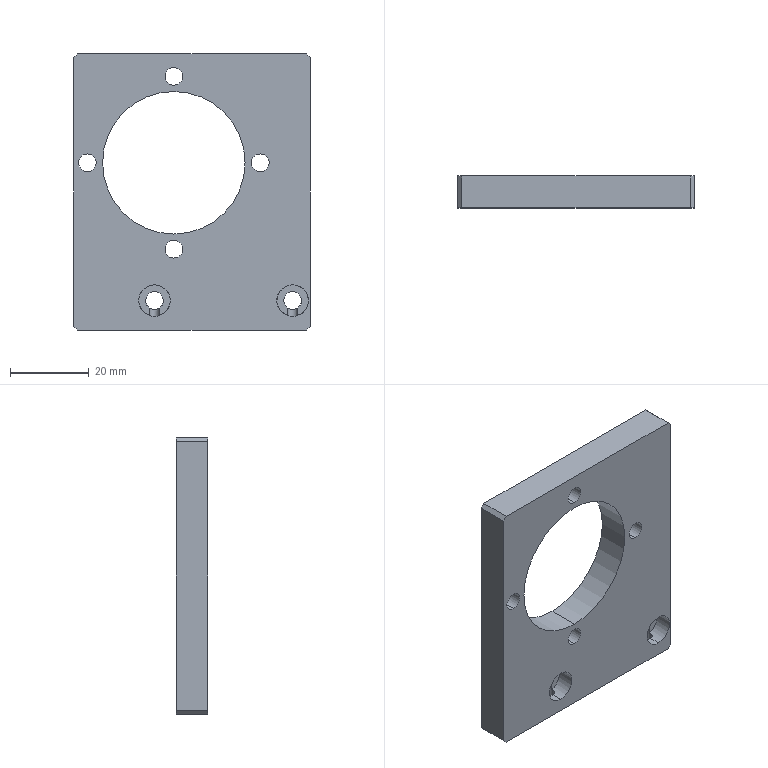Part | STEP file | 08-19 rotary cylinder mounting plate | 1 solid | 34 faces | box 60 x 8 x 70 mm | volume 24290 mm3 | cylinder 22 | plane 12 | commonest cylinder face diameters 4.5 x12 2.5 x4 8 x4 36.1 x2
STEP:
#1=CARTESIAN_POINT('',(26.75,0.,-31.3));
#2=VERTEX_POINT('',#1);
#3=CARTESIAN_POINT('',(25.5,-1.25,-31.5));
#4=VERTEX_POINT('',#3);
#5=CARTESIAN_POINT('',(26.75,0.,-31.3));
#6=CARTESIAN_POINT('',(26.75,-0.1662,-31.3));
#7=CARTESIAN_POINT('',(26.717,-0.3296,-31.311));
#8=CARTESIAN_POINT('',(26.591,-0.6317,-31.349));
#9=CARTESIAN_POINT('',(26.498,-0.7698,-31.375));
#10=CARTESIAN_POINT('',(26.269,-0.9987,-31.427));
#11=CARTESIAN_POINT('',(26.13,-1.092,-31.453));
#12=CARTESIAN_POINT('',(25.83,-1.217,-31.489));
#13=CARTESIAN_POINT('',(25.664,-1.25,-31.5));
#14=CARTESIAN_POINT('',(25.5,-1.25,-31.5));
#15=B_SPLINE_CURVE_WITH_KNOTS('',3,(#5,#6,#7,#8,#9,#10,#11,#12,#13,#14),.UNSPECIFIED.,.F.,.F.,(4,2,2,2,4),(0.0004059,0.0008978,0.00139,0.001882,0.002374),.UNSPECIFIED.);
#16=EDGE_CURVE('',#2,#4,#15,.T.);
#17=ORIENTED_EDGE('',*,*,#16,.F.);
#18=CARTESIAN_POINT('',(26.75,0.,-35.));
#19=VERTEX_POINT('',#18);
#20=CARTESIAN_POINT('',(26.75,0.,-35.));
#21=DIRECTION('',(0.,0.,-1.));
#22=VECTOR('',#21,1000.);
#23=LINE('',#20,#22);
#24=EDGE_CURVE('',#2,#19,#23,.T.);
#25=ORIENTED_EDGE('',*,*,#24,.T.);
#26=CARTESIAN_POINT('',(24.25,0.,-35.));
#27=VERTEX_POINT('',#26);
#28=CARTESIAN_POINT('',(25.5,0.,-35.));
#29=DIRECTION('',(0.,0.,-1.));
#30=DIRECTION('',(-1.,0.,0.));
#31=AXIS2_PLACEMENT_3D('',#28,#29,#30);
#32=CIRCLE('',#31,1.25);
#33=EDGE_CURVE('',#19,#27,#32,.T.);
#34=ORIENTED_EDGE('',*,*,#33,.T.);
#35=CARTESIAN_POINT('',(24.25,0.,-31.3));
#36=VERTEX_POINT('',#35);
#37=CARTESIAN_POINT('',(24.25,0.,-35.));
#38=DIRECTION('',(0.,0.,-1.));
#39=VECTOR('',#38,1000.);
#40=LINE('',#37,#39);
#41=EDGE_CURVE('',#36,#27,#40,.T.);
#42=ORIENTED_EDGE('',*,*,#41,.F.);
#43=CARTESIAN_POINT('',(25.5,-1.25,-31.5));
#44=CARTESIAN_POINT('',(25.418,-1.25,-31.5));
#45=CARTESIAN_POINT('',(25.334,-1.242,-31.497));
#46=CARTESIAN_POINT('',(25.174,-1.209,-31.487));
#47=CARTESIAN_POINT('',(25.096,-1.186,-31.48));
#48=CARTESIAN_POINT('',(24.867,-1.091,-31.453));
#49=CARTESIAN_POINT('',(24.73,-0.9983,-31.427));
#50=CARTESIAN_POINT('',(24.558,-0.8256,-31.388));
#51=CARTESIAN_POINT('',(24.507,-0.763,-31.375));
#52=CARTESIAN_POINT('',(24.416,-0.6278,-31.351));
#53=CARTESIAN_POINT('',(24.377,-0.5547,-31.339));
#54=CARTESIAN_POINT('',(24.283,-0.3291,-31.311));
#55=CARTESIAN_POINT('',(24.25,-0.1638,-31.3));
#56=CARTESIAN_POINT('',(24.25,0.,-31.3));
#57=B_SPLINE_CURVE_WITH_KNOTS('',3,(#43,#44,#45,#46,#47,#48,#49,#50,#51,#52,#53,#54,#55,#56),.UNSPECIFIED.,.F.,.F.,(4,2,2,2,2,2,4),(0.002374,0.002619,0.002865,0.003357,0.003603,0.003849,0.00434),.UNSPECIFIED.);
#58=EDGE_CURVE('',#4,#36,#57,.T.);
#59=ORIENTED_EDGE('',*,*,#58,.F.);
#60=EDGE_LOOP('',(#17,#25,#34,#42,#59));
#61=FACE_OUTER_BOUND('',#60,.T.);
#62=CARTESIAN_POINT('',(25.5,0.,-35.));
#63=DIRECTION('',(0.,0.,-1.));
#64=DIRECTION('',(-1.,0.,0.));
#65=AXIS2_PLACEMENT_3D('',#62,#63,#64);
#66=CYLINDRICAL_SURFACE('',#65,1.25);
#67=ADVANCED_FACE('',(#61),#66,.F.);
#68=CARTESIAN_POINT('',(-8.25,0.,-31.3));
#69=VERTEX_POINT('',#68);
#70=CARTESIAN_POINT('',(-9.5,-1.25,-31.5));
#71=VERTEX_POINT('',#70);
#72=CARTESIAN_POINT('',(-8.25,0.,-31.3));
#73=CARTESIAN_POINT('',(-8.25,-0.1662,-31.3));
#74=CARTESIAN_POINT('',(-8.283,-0.3296,-31.311));
#75=CARTESIAN_POINT('',(-8.409,-0.6317,-31.349));
#76=CARTESIAN_POINT('',(-8.502,-0.7698,-31.375));
#77=CARTESIAN_POINT('',(-8.731,-0.9987,-31.427));
#78=CARTESIAN_POINT('',(-8.87,-1.092,-31.453));
#79=CARTESIAN_POINT('',(-9.17,-1.217,-31.489));
#80=CARTESIAN_POINT('',(-9.336,-1.25,-31.5));
#81=CARTESIAN_POINT('',(-9.5,-1.25,-31.5));
#82=B_SPLINE_CURVE_WITH_KNOTS('',3,(#72,#73,#74,#75,#76,#77,#78,#79,#80,#81),.UNSPECIFIED.,.F.,.F.,(4,2,2,2,4),(0.0004059,0.0008978,0.00139,0.001882,0.002374),.UNSPECIFIED.);
#83=EDGE_CURVE('',#69,#71,#82,.T.);
#84=ORIENTED_EDGE('',*,*,#83,.F.);
#85=CARTESIAN_POINT('',(-8.25,0.,-35.));
#86=VERTEX_POINT('',#85);
#87=CARTESIAN_POINT('',(-8.25,0.,-35.));
#88=DIRECTION('',(0.,0.,-1.));
#89=VECTOR('',#88,1000.);
#90=LINE('',#87,#89);
#91=EDGE_CURVE('',#69,#86,#90,.T.);
#92=ORIENTED_EDGE('',*,*,#91,.T.);
#93=CARTESIAN_POINT('',(-10.75,0.,-35.));
#94=VERTEX_POINT('',#93);
#95=CARTESIAN_POINT('',(-9.5,0.,-35.));
#96=DIRECTION('',(0.,0.,-1.));
#97=DIRECTION('',(-1.,0.,0.));
#98=AXIS2_PLACEMENT_3D('',#95,#96,#97);
#99=CIRCLE('',#98,1.25);
#100=EDGE_CURVE('',#86,#94,#99,.T.);
#101=ORIENTED_EDGE('',*,*,#100,.T.);
#102=CARTESIAN_POINT('',(-10.75,0.,-31.3));
#103=VERTEX_POINT('',#102);
#104=CARTESIAN_POINT('',(-10.75,0.,-35.));
#105=DIRECTION('',(0.,0.,-1.));
#106=VECTOR('',#105,1000.);
#107=LINE('',#104,#106);
#108=EDGE_CURVE('',#103,#94,#107,.T.);
#109=ORIENTED_EDGE('',*,*,#108,.F.);
#110=CARTESIAN_POINT('',(-9.5,-1.25,-31.5));
#111=CARTESIAN_POINT('',(-9.582,-1.25,-31.5));
#112=CARTESIAN_POINT('',(-9.666,-1.242,-31.497));
#113=CARTESIAN_POINT('',(-9.826,-1.209,-31.487));
#114=CARTESIAN_POINT('',(-9.904,-1.186,-31.48));
#115=CARTESIAN_POINT('',(-10.133,-1.091,-31.453));
#116=CARTESIAN_POINT('',(-10.27,-0.9983,-31.427));
#117=CARTESIAN_POINT('',(-10.442,-0.8256,-31.388));
#118=CARTESIAN_POINT('',(-10.493,-0.763,-31.375));
#119=CARTESIAN_POINT('',(-10.584,-0.6278,-31.351));
#120=CARTESIAN_POINT('',(-10.623,-0.5547,-31.339));
#121=CARTESIAN_POINT('',(-10.717,-0.3291,-31.311));
#122=CARTESIAN_POINT('',(-10.75,-0.1638,-31.3));
#123=CARTESIAN_POINT('',(-10.75,0.,-31.3));
#124=B_SPLINE_CURVE_WITH_KNOTS('',3,(#110,#111,#112,#113,#114,#115,#116,#117,#118,#119,#120,#121,#122,#123),.UNSPECIFIED.,.F.,.F.,(4,2,2,2,2,2,4),(0.002374,0.002619,0.002865,0.003357,0.003603,0.003849,0.00434),.UNSPECIFIED.);
#125=EDGE_CURVE('',#71,#103,#124,.T.);
#126=ORIENTED_EDGE('',*,*,#125,.F.);
#127=EDGE_LOOP('',(#84,#92,#101,#109,#126));
#128=FACE_OUTER_BOUND('',#127,.T.);
#129=CARTESIAN_POINT('',(-9.5,0.,-35.));
#130=DIRECTION('',(0.,0.,-1.));
#131=DIRECTION('',(-1.,0.,0.));
#132=AXIS2_PLACEMENT_3D('',#129,#130,#131);
#133=CYLINDRICAL_SURFACE('',#132,1.25);
#134=ADVANCED_FACE('',(#128),#133,.F.);
#135=CARTESIAN_POINT('',(-9.5,0.4,-23.5));
#136=VERTEX_POINT('',#135);
#137=CARTESIAN_POINT('',(-10.684,0.4,-31.321));
#138=VERTEX_POINT('',#137);
#139=CARTESIAN_POINT('',(-9.5,0.4,-27.5));
#140=DIRECTION('',(0.,-1.,0.));
#141=DIRECTION('',(0.,0.,-1.));
#142=AXIS2_PLACEMENT_3D('',#139,#140,#141);
#143=CIRCLE('',#142,4.);
#144=EDGE_CURVE('',#136,#138,#143,.T.);
#145=ORIENTED_EDGE('',*,*,#144,.F.);
#146=CARTESIAN_POINT('',(-9.5,-4.,-23.5));
#147=VERTEX_POINT('',#146);
#148=CARTESIAN_POINT('',(-9.5,-4.,-23.5));
#149=DIRECTION('',(0.,-1.,0.));
#150=VECTOR('',#149,1000.);
#151=LINE('',#148,#150);
#152=EDGE_CURVE('',#136,#147,#151,.T.);
#153=ORIENTED_EDGE('',*,*,#152,.T.);
#154=CARTESIAN_POINT('',(-9.5,-4.,-31.5));
#155=VERTEX_POINT('',#154);
#156=CARTESIAN_POINT('',(-9.5,-4.,-27.5));
#157=DIRECTION('',(0.,-1.,0.));
#158=DIRECTION('',(0.,0.,-1.));
#159=AXIS2_PLACEMENT_3D('',#156,#157,#158);
#160=CIRCLE('',#159,4.);
#161=EDGE_CURVE('',#147,#155,#160,.T.);
#162=ORIENTED_EDGE('',*,*,#161,.T.);
#163=CARTESIAN_POINT('',(-9.5,-4.,-31.5));
#164=DIRECTION('',(0.,-1.,0.));
#165=VECTOR('',#164,1000.);
#166=LINE('',#163,#165);
#167=EDGE_CURVE('',#71,#155,#166,.T.);
#168=ORIENTED_EDGE('',*,*,#167,.F.);
#169=ORIENTED_EDGE('',*,*,#125,.T.);
#170=CARTESIAN_POINT('',(-10.75,0.,-31.3));
#171=CARTESIAN_POINT('',(-10.75,0.1348,-31.3));
#172=CARTESIAN_POINT('',(-10.728,0.271,-31.307));
#173=CARTESIAN_POINT('',(-10.684,0.4,-31.321));
#174=B_SPLINE_CURVE_WITH_KNOTS('',3,(#170,#171,#172,#173),.UNSPECIFIED.,.F.,.F.,(4,4),(0.00434,0.004745),.UNSPECIFIED.);
#175=EDGE_CURVE('',#103,#138,#174,.T.);
#176=ORIENTED_EDGE('',*,*,#175,.T.);
#177=EDGE_LOOP('',(#145,#153,#162,#168,#169,#176));
#178=FACE_OUTER_BOUND('',#177,.T.);
#179=CARTESIAN_POINT('',(-9.5,-4.,-27.5));
#180=DIRECTION('',(0.,-1.,0.));
#181=DIRECTION('',(0.,0.,-1.));
#182=AXIS2_PLACEMENT_3D('',#179,#180,#181);
#183=CYLINDRICAL_SURFACE('',#182,4.);
#184=ADVANCED_FACE('',(#178),#183,.F.);
#185=CARTESIAN_POINT('',(-9.5,4.,-25.25));
#186=VERTEX_POINT('',#185);
#187=CARTESIAN_POINT('',(-9.5,4.,-29.75));
#188=VERTEX_POINT('',#187);
#189=CARTESIAN_POINT('',(-9.5,4.,-27.5));
#190=DIRECTION('',(0.,-1.,0.));
#191=DIRECTION('',(0.,0.,-1.));
#192=AXIS2_PLACEMENT_3D('',#189,#190,#191);
#193=CIRCLE('',#192,2.25);
#194=EDGE_CURVE('',#186,#188,#193,.T.);
#195=ORIENTED_EDGE('',*,*,#194,.F.);
#196=CARTESIAN_POINT('',(-9.5,0.4,-25.25));
#197=VERTEX_POINT('',#196);
#198=CARTESIAN_POINT('',(-9.5,-4.,-25.25));
#199=DIRECTION('',(0.,-1.,0.));
#200=VECTOR('',#199,1000.);
#201=LINE('',#198,#200);
#202=EDGE_CURVE('',#186,#197,#201,.T.);
#203=ORIENTED_EDGE('',*,*,#202,.T.);
#204=CARTESIAN_POINT('',(-10.684,0.4,-29.413));
#205=VERTEX_POINT('',#204);
#206=CARTESIAN_POINT('',(-9.5,0.4,-27.5));
#207=DIRECTION('',(0.,-1.,0.));
#208=DIRECTION('',(0.,0.,-1.));
#209=AXIS2_PLACEMENT_3D('',#206,#207,#208);
#210=CIRCLE('',#209,2.25);
#211=EDGE_CURVE('',#197,#205,#210,.T.);
#212=ORIENTED_EDGE('',*,*,#211,.T.);
#213=CARTESIAN_POINT('',(-9.5,1.25,-29.75));
#214=VERTEX_POINT('',#213);
#215=CARTESIAN_POINT('',(-10.684,0.4,-29.413));
#216=CARTESIAN_POINT('',(-10.642,0.5252,-29.439));
#217=CARTESIAN_POINT('',(-10.582,0.6383,-29.474));
#218=CARTESIAN_POINT('',(-10.43,0.8448,-29.55));
#219=CARTESIAN_POINT('',(-10.339,0.935,-29.59));
#220=CARTESIAN_POINT('',(-10.132,1.086,-29.662));
#221=CARTESIAN_POINT('',(-10.015,1.146,-29.694));
#222=CARTESIAN_POINT('',(-9.767,1.228,-29.738));
#223=CARTESIAN_POINT('',(-9.633,1.25,-29.75));
#224=CARTESIAN_POINT('',(-9.5,1.25,-29.75));
#225=B_SPLINE_CURVE_WITH_KNOTS('',3,(#215,#216,#217,#218,#219,#220,#221,#222,#223,#224),.UNSPECIFIED.,.F.,.F.,(4,2,2,2,4),(0.,0.0003977,0.0007954,0.001193,0.001591),.UNSPECIFIED.);
#226=EDGE_CURVE('',#205,#214,#225,.T.);
#227=ORIENTED_EDGE('',*,*,#226,.T.);
#228=CARTESIAN_POINT('',(-9.5,-4.,-29.75));
#229=DIRECTION('',(0.,-1.,0.));
#230=VECTOR('',#229,1000.);
#231=LINE('',#228,#230);
#232=EDGE_CURVE('',#188,#214,#231,.T.);
#233=ORIENTED_EDGE('',*,*,#232,.F.);
#234=EDGE_LOOP('',(#195,#203,#212,#227,#233));
#235=FACE_OUTER_BOUND('',#234,.T.);
#236=CARTESIAN_POINT('',(-9.5,-4.,-27.5));
#237=DIRECTION('',(0.,-1.,0.));
#238=DIRECTION('',(0.,0.,-1.));
#239=AXIS2_PLACEMENT_3D('',#236,#237,#238);
#240=CYLINDRICAL_SURFACE('',#239,2.25);
#241=ADVANCED_FACE('',(#235),#240,.F.);
#242=CARTESIAN_POINT('',(25.5,0.4,-23.5));
#243=VERTEX_POINT('',#242);
#244=CARTESIAN_POINT('',(24.316,0.4,-31.321));
#245=VERTEX_POINT('',#244);
#246=CARTESIAN_POINT('',(25.5,0.4,-27.5));
#247=DIRECTION('',(0.,-1.,0.));
#248=DIRECTION('',(0.,0.,-1.));
#249=AXIS2_PLACEMENT_3D('',#246,#247,#248);
#250=CIRCLE('',#249,4.);
#251=EDGE_CURVE('',#243,#245,#250,.T.);
#252=ORIENTED_EDGE('',*,*,#251,.F.);
#253=CARTESIAN_POINT('',(25.5,-4.,-23.5));
#254=VERTEX_POINT('',#253);
#255=CARTESIAN_POINT('',(25.5,-4.,-23.5));
#256=DIRECTION('',(0.,-1.,0.));
#257=VECTOR('',#256,1000.);
#258=LINE('',#255,#257);
#259=EDGE_CURVE('',#243,#254,#258,.T.);
#260=ORIENTED_EDGE('',*,*,#259,.T.);
#261=CARTESIAN_POINT('',(25.5,-4.,-31.5));
#262=VERTEX_POINT('',#261);
#263=CARTESIAN_POINT('',(25.5,-4.,-27.5));
#264=DIRECTION('',(0.,-1.,0.));
#265=DIRECTION('',(0.,0.,-1.));
#266=AXIS2_PLACEMENT_3D('',#263,#264,#265);
#267=CIRCLE('',#266,4.);
#268=EDGE_CURVE('',#254,#262,#267,.T.);
#269=ORIENTED_EDGE('',*,*,#268,.T.);
#270=CARTESIAN_POINT('',(25.5,-4.,-31.5));
#271=DIRECTION('',(0.,-1.,0.));
#272=VECTOR('',#271,1000.);
#273=LINE('',#270,#272);
#274=EDGE_CURVE('',#4,#262,#273,.T.);
#275=ORIENTED_EDGE('',*,*,#274,.F.);
#276=ORIENTED_EDGE('',*,*,#58,.T.);
#277=CARTESIAN_POINT('',(24.25,0.,-31.3));
#278=CARTESIAN_POINT('',(24.25,0.1348,-31.3));
#279=CARTESIAN_POINT('',(24.272,0.271,-31.307));
#280=CARTESIAN_POINT('',(24.316,0.4,-31.321));
#281=B_SPLINE_CURVE_WITH_KNOTS('',3,(#277,#278,#279,#280),.UNSPECIFIED.,.F.,.F.,(4,4),(0.00434,0.004745),.UNSPECIFIED.);
#282=EDGE_CURVE('',#36,#245,#281,.T.);
#283=ORIENTED_EDGE('',*,*,#282,.T.);
#284=EDGE_LOOP('',(#252,#260,#269,#275,#276,#283));
#285=FACE_OUTER_BOUND('',#284,.T.);
#286=CARTESIAN_POINT('',(25.5,-4.,-27.5));
#287=DIRECTION('',(0.,-1.,0.));
#288=DIRECTION('',(0.,0.,-1.));
#289=AXIS2_PLACEMENT_3D('',#286,#287,#288);
#290=CYLINDRICAL_SURFACE('',#289,4.);
#291=ADVANCED_FACE('',(#285),#290,.F.);
#292=CARTESIAN_POINT('',(25.5,4.,-25.25));
#293=VERTEX_POINT('',#292);
#294=CARTESIAN_POINT('',(25.5,4.,-29.75));
#295=VERTEX_POINT('',#294);
#296=CARTESIAN_POINT('',(25.5,4.,-27.5));
#297=DIRECTION('',(0.,-1.,0.));
#298=DIRECTION('',(0.,0.,-1.));
#299=AXIS2_PLACEMENT_3D('',#296,#297,#298);
#300=CIRCLE('',#299,2.25);
#301=EDGE_CURVE('',#293,#295,#300,.T.);
#302=ORIENTED_EDGE('',*,*,#301,.F.);
#303=CARTESIAN_POINT('',(25.5,0.4,-25.25));
#304=VERTEX_POINT('',#303);
#305=CARTESIAN_POINT('',(25.5,-4.,-25.25));
#306=DIRECTION('',(0.,-1.,0.));
#307=VECTOR('',#306,1000.);
#308=LINE('',#305,#307);
#309=EDGE_CURVE('',#293,#304,#308,.T.);
#310=ORIENTED_EDGE('',*,*,#309,.T.);
#311=CARTESIAN_POINT('',(24.316,0.4,-29.413));
#312=VERTEX_POINT('',#311);
#313=CARTESIAN_POINT('',(25.5,0.4,-27.5));
#314=DIRECTION('',(0.,-1.,0.));
#315=DIRECTION('',(0.,0.,-1.));
#316=AXIS2_PLACEMENT_3D('',#313,#314,#315);
#317=CIRCLE('',#316,2.25);
#318=EDGE_CURVE('',#304,#312,#317,.T.);
#319=ORIENTED_EDGE('',*,*,#318,.T.);
#320=CARTESIAN_POINT('',(25.5,1.25,-29.75));
#321=VERTEX_POINT('',#320);
#322=CARTESIAN_POINT('',(24.316,0.4,-29.413));
#323=CARTESIAN_POINT('',(24.358,0.5252,-29.439));
#324=CARTESIAN_POINT('',(24.418,0.6383,-29.474));
#325=CARTESIAN_POINT('',(24.57,0.8448,-29.55));
#326=CARTESIAN_POINT('',(24.661,0.935,-29.59));
#327=CARTESIAN_POINT('',(24.868,1.086,-29.662));
#328=CARTESIAN_POINT('',(24.985,1.146,-29.694));
#329=CARTESIAN_POINT('',(25.233,1.228,-29.738));
#330=CARTESIAN_POINT('',(25.367,1.25,-29.75));
#331=CARTESIAN_POINT('',(25.5,1.25,-29.75));
#332=B_SPLINE_CURVE_WITH_KNOTS('',3,(#322,#323,#324,#325,#326,#327,#328,#329,#330,#331),.UNSPECIFIED.,.F.,.F.,(4,2,2,2,4),(0.,0.0003977,0.0007954,0.001193,0.001591),.UNSPECIFIED.);
#333=EDGE_CURVE('',#312,#321,#332,.T.);
#334=ORIENTED_EDGE('',*,*,#333,.T.);
#335=CARTESIAN_POINT('',(25.5,-4.,-29.75));
#336=DIRECTION('',(0.,-1.,0.));
#337=VECTOR('',#336,1000.);
#338=LINE('',#335,#337);
#339=EDGE_CURVE('',#295,#321,#338,.T.);
#340=ORIENTED_EDGE('',*,*,#339,.F.);
#341=EDGE_LOOP('',(#302,#310,#319,#334,#340));
#342=FACE_OUTER_BOUND('',#341,.T.);
#343=CARTESIAN_POINT('',(25.5,-4.,-27.5));
#344=DIRECTION('',(0.,-1.,0.));
#345=DIRECTION('',(0.,0.,-1.));
#346=AXIS2_PLACEMENT_3D('',#343,#344,#345);
#347=CYLINDRICAL_SURFACE('',#346,2.25);
#348=ADVANCED_FACE('',(#342),#347,.F.);
#349=CARTESIAN_POINT('',(17.3,4.,5.15));
#350=VERTEX_POINT('',#349);
#351=CARTESIAN_POINT('',(17.3,4.,9.65));
#352=VERTEX_POINT('',#351);
#353=CARTESIAN_POINT('',(17.3,4.,7.4));
#354=DIRECTION('',(0.,1.,0.));
#355=DIRECTION('',(0.,0.,1.));
#356=AXIS2_PLACEMENT_3D('',#353,#354,#355);
#357=CIRCLE('',#356,2.25);
#358=EDGE_CURVE('',#350,#352,#357,.T.);
#359=ORIENTED_EDGE('',*,*,#358,.T.);
#360=CARTESIAN_POINT('',(17.3,-4.,9.65));
#361=VERTEX_POINT('',#360);
#362=CARTESIAN_POINT('',(17.3,6.,9.65));
#363=DIRECTION('',(0.,-1.,0.));
#364=VECTOR('',#363,1000.);
#365=LINE('',#362,#364);
#366=EDGE_CURVE('',#352,#361,#365,.T.);
#367=ORIENTED_EDGE('',*,*,#366,.T.);
#368=CARTESIAN_POINT('',(17.3,-4.,5.15));
#369=VERTEX_POINT('',#368);
#370=CARTESIAN_POINT('',(17.3,-4.,7.4));
#371=DIRECTION('',(0.,-1.,0.));
#372=DIRECTION('',(1.,0.,0.));
#373=AXIS2_PLACEMENT_3D('',#370,#371,#372);
#374=CIRCLE('',#373,2.25);
#375=EDGE_CURVE('',#361,#369,#374,.T.);
#376=ORIENTED_EDGE('',*,*,#375,.T.);
#377=CARTESIAN_POINT('',(17.3,6.,5.15));
#378=DIRECTION('',(0.,-1.,0.));
#379=VECTOR('',#378,1000.);
#380=LINE('',#377,#379);
#381=EDGE_CURVE('',#350,#369,#380,.T.);
#382=ORIENTED_EDGE('',*,*,#381,.F.);
#383=EDGE_LOOP('',(#359,#367,#376,#382));
#384=FACE_OUTER_BOUND('',#383,.T.);
#385=CARTESIAN_POINT('',(17.3,6.,7.4));
#386=DIRECTION('',(0.,-1.,0.));
#387=DIRECTION('',(0.,0.,-1.));
#388=AXIS2_PLACEMENT_3D('',#385,#386,#387);
#389=CYLINDRICAL_SURFACE('',#388,2.25);
#390=ADVANCED_FACE('',(#384),#389,.F.);
#391=CARTESIAN_POINT('',(-26.5,4.,5.15));
#392=VERTEX_POINT('',#391);
#393=CARTESIAN_POINT('',(-26.5,4.,9.65));
#394=VERTEX_POINT('',#393);
#395=CARTESIAN_POINT('',(-26.5,4.,7.4));
#396=DIRECTION('',(0.,1.,0.));
#397=DIRECTION('',(0.,0.,1.));
#398=AXIS2_PLACEMENT_3D('',#395,#396,#397);
#399=CIRCLE('',#398,2.25);
#400=EDGE_CURVE('',#392,#394,#399,.T.);
#401=ORIENTED_EDGE('',*,*,#400,.T.);
#402=CARTESIAN_POINT('',(-26.5,-4.,9.65));
#403=VERTEX_POINT('',#402);
#404=CARTESIAN_POINT('',(-26.5,6.,9.65));
#405=DIRECTION('',(0.,-1.,0.));
#406=VECTOR('',#405,1000.);
#407=LINE('',#404,#406);
#408=EDGE_CURVE('',#394,#403,#407,.T.);
#409=ORIENTED_EDGE('',*,*,#408,.T.);
#410=CARTESIAN_POINT('',(-26.5,-4.,5.15));
#411=VERTEX_POINT('',#410);
#412=CARTESIAN_POINT('',(-26.5,-4.,7.4));
#413=DIRECTION('',(0.,-1.,0.));
#414=DIRECTION('',(1.,0.,0.));
#415=AXIS2_PLACEMENT_3D('',#412,#413,#414);
#416=CIRCLE('',#415,2.25);
#417=EDGE_CURVE('',#403,#411,#416,.T.);
#418=ORIENTED_EDGE('',*,*,#417,.T.);
#419=CARTESIAN_POINT('',(-26.5,6.,5.15));
#420=DIRECTION('',(0.,-1.,0.));
#421=VECTOR('',#420,1000.);
#422=LINE('',#419,#421);
#423=EDGE_CURVE('',#392,#411,#422,.T.);
#424=ORIENTED_EDGE('',*,*,#423,.F.);
#425=EDGE_LOOP('',(#401,#409,#418,#424));
#426=FACE_OUTER_BOUND('',#425,.T.);
#427=CARTESIAN_POINT('',(-26.5,6.,7.4));
#428=DIRECTION('',(0.,-1.,0.));
#429=DIRECTION('',(0.,0.,-1.));
#430=AXIS2_PLACEMENT_3D('',#427,#428,#429);
#431=CYLINDRICAL_SURFACE('',#430,2.25);
#432=ADVANCED_FACE('',(#426),#431,.F.);
#433=CARTESIAN_POINT('',(-4.6,4.,-16.75));
#434=VERTEX_POINT('',#433);
#435=CARTESIAN_POINT('',(-4.6,4.,-12.25));
#436=VERTEX_POINT('',#435);
#437=CARTESIAN_POINT('',(-4.6,4.,-14.5));
#438=DIRECTION('',(0.,1.,0.));
#439=DIRECTION('',(0.,0.,1.));
#440=AXIS2_PLACEMENT_3D('',#437,#438,#439);
#441=CIRCLE('',#440,2.25);
#442=EDGE_CURVE('',#434,#436,#441,.T.);
#443=ORIENTED_EDGE('',*,*,#442,.T.);
#444=CARTESIAN_POINT('',(-4.6,-4.,-12.25));
#445=VERTEX_POINT('',#444);
#446=CARTESIAN_POINT('',(-4.6,6.,-12.25));
#447=DIRECTION('',(0.,-1.,0.));
#448=VECTOR('',#447,1000.);
#449=LINE('',#446,#448);
#450=EDGE_CURVE('',#436,#445,#449,.T.);
#451=ORIENTED_EDGE('',*,*,#450,.T.);
#452=CARTESIAN_POINT('',(-4.6,-4.,-16.75));
#453=VERTEX_POINT('',#452);
#454=CARTESIAN_POINT('',(-4.6,-4.,-14.5));
#455=DIRECTION('',(0.,-1.,0.));
#456=DIRECTION('',(0.,0.,-1.));
#457=AXIS2_PLACEMENT_3D('',#454,#455,#456);
#458=CIRCLE('',#457,2.25);
#459=EDGE_CURVE('',#445,#453,#458,.T.);
#460=ORIENTED_EDGE('',*,*,#459,.T.);
#461=CARTESIAN_POINT('',(-4.6,6.,-16.75));
#462=DIRECTION('',(0.,-1.,0.));
#463=VECTOR('',#462,1000.);
#464=LINE('',#461,#463);
#465=EDGE_CURVE('',#434,#453,#464,.T.);
#466=ORIENTED_EDGE('',*,*,#465,.F.);
#467=EDGE_LOOP('',(#443,#451,#460,#466));
#468=FACE_OUTER_BOUND('',#467,.T.);
#469=CARTESIAN_POINT('',(-4.6,6.,-14.5));
#470=DIRECTION('',(0.,-1.,0.));
#471=DIRECTION('',(0.,0.,-1.));
#472=AXIS2_PLACEMENT_3D('',#469,#470,#471);
#473=CYLINDRICAL_SURFACE('',#472,2.25);
#474=ADVANCED_FACE('',(#468),#473,.F.);
#475=CARTESIAN_POINT('',(-4.6,4.,27.05));
#476=VERTEX_POINT('',#475);
#477=CARTESIAN_POINT('',(-4.6,4.,31.55));
#478=VERTEX_POINT('',#477);
#479=CARTESIAN_POINT('',(-4.6,4.,29.3));
#480=DIRECTION('',(0.,1.,0.));
#481=DIRECTION('',(0.,0.,1.));
#482=AXIS2_PLACEMENT_3D('',#479,#480,#481);
#483=CIRCLE('',#482,2.25);
#484=EDGE_CURVE('',#476,#478,#483,.T.);
#485=ORIENTED_EDGE('',*,*,#484,.T.);
#486=CARTESIAN_POINT('',(-4.6,-4.,31.55));
#487=VERTEX_POINT('',#486);
#488=CARTESIAN_POINT('',(-4.6,6.,31.55));
#489=DIRECTION('',(0.,-1.,0.));
#490=VECTOR('',#489,1000.);
#491=LINE('',#488,#490);
#492=EDGE_CURVE('',#478,#487,#491,.T.);
#493=ORIENTED_EDGE('',*,*,#492,.T.);
#494=CARTESIAN_POINT('',(-4.6,-4.,27.05));
#495=VERTEX_POINT('',#494);
#496=CARTESIAN_POINT('',(-4.6,-4.,29.3));
#497=DIRECTION('',(0.,-1.,0.));
#498=DIRECTION('',(0.,0.,-1.));
#499=AXIS2_PLACEMENT_3D('',#496,#497,#498);
#500=CIRCLE('',#499,2.25);
#501=EDGE_CURVE('',#487,#495,#500,.T.);
#502=ORIENTED_EDGE('',*,*,#501,.T.);
#503=CARTESIAN_POINT('',(-4.6,6.,27.05));
#504=DIRECTION('',(0.,-1.,0.));
#505=VECTOR('',#504,1000.);
#506=LINE('',#503,#505);
#507=EDGE_CURVE('',#476,#495,#506,.T.);
#508=ORIENTED_EDGE('',*,*,#507,.F.);
#509=EDGE_LOOP('',(#485,#493,#502,#508));
#510=FACE_OUTER_BOUND('',#509,.T.);
#511=CARTESIAN_POINT('',(-4.6,6.,29.3));
#512=DIRECTION('',(0.,-1.,0.));
#513=DIRECTION('',(0.,0.,-1.));
#514=AXIS2_PLACEMENT_3D('',#511,#512,#513);
#515=CYLINDRICAL_SURFACE('',#514,2.25);
#516=ADVANCED_FACE('',(#510),#515,.F.);
#517=CARTESIAN_POINT('',(-4.6,4.,-10.65));
#518=VERTEX_POINT('',#517);
#519=CARTESIAN_POINT('',(-4.6,4.,25.45));
#520=VERTEX_POINT('',#519);
#521=CARTESIAN_POINT('',(-4.6,4.,7.4));
#522=DIRECTION('',(0.,1.,0.));
#523=DIRECTION('',(0.,0.,1.));
#524=AXIS2_PLACEMENT_3D('',#521,#522,#523);
#525=CIRCLE('',#524,18.05);
#526=EDGE_CURVE('',#518,#520,#525,.T.);
#527=ORIENTED_EDGE('',*,*,#526,.T.);
#528=CARTESIAN_POINT('',(-4.6,-4.,25.45));
#529=VERTEX_POINT('',#528);
#530=CARTESIAN_POINT('',(-4.6,6.,25.45));
#531=DIRECTION('',(0.,-1.,0.));
#532=VECTOR('',#531,1000.);
#533=LINE('',#530,#532);
#534=EDGE_CURVE('',#520,#529,#533,.T.);
#535=ORIENTED_EDGE('',*,*,#534,.T.);
#536=CARTESIAN_POINT('',(-4.6,-4.,-10.65));
#537=VERTEX_POINT('',#536);
#538=CARTESIAN_POINT('',(-4.6,-4.,7.4));
#539=DIRECTION('',(0.,-1.,0.));
#540=DIRECTION('',(0.,0.,-1.));
#541=AXIS2_PLACEMENT_3D('',#538,#539,#540);
#542=CIRCLE('',#541,18.05);
#543=EDGE_CURVE('',#529,#537,#542,.T.);
#544=ORIENTED_EDGE('',*,*,#543,.T.);
#545=CARTESIAN_POINT('',(-4.6,6.,-10.65));
#546=DIRECTION('',(0.,-1.,0.));
#547=VECTOR('',#546,1000.);
#548=LINE('',#545,#547);
#549=EDGE_CURVE('',#518,#537,#548,.T.);
#550=ORIENTED_EDGE('',*,*,#549,.F.);
#551=EDGE_LOOP('',(#527,#535,#544,#550));
#552=FACE_OUTER_BOUND('',#551,.T.);
#553=CARTESIAN_POINT('',(-4.6,6.,7.4));
#554=DIRECTION('',(0.,-1.,0.));
#555=DIRECTION('',(0.,0.,-1.));
#556=AXIS2_PLACEMENT_3D('',#553,#554,#555);
#557=CYLINDRICAL_SURFACE('',#556,18.05);
#558=ADVANCED_FACE('',(#552),#557,.F.);
#559=CARTESIAN_POINT('',(30.,-4.,34.));
#560=VERTEX_POINT('',#559);
#561=CARTESIAN_POINT('',(30.,-4.,-34.));
#562=VERTEX_POINT('',#561);
#563=CARTESIAN_POINT('',(30.,-4.,-35.));
#564=DIRECTION('',(0.,0.,-1.));
#565=VECTOR('',#564,1000.);
#566=LINE('',#563,#565);
#567=EDGE_CURVE('',#560,#562,#566,.T.);
#568=ORIENTED_EDGE('',*,*,#567,.T.);
#569=CARTESIAN_POINT('',(30.,4.,-34.));
#570=VERTEX_POINT('',#569);
#571=CARTESIAN_POINT('',(30.,4.,-34.));
#572=DIRECTION('',(0.,1.,0.));
#573=VECTOR('',#572,1000.);
#574=LINE('',#571,#573);
#575=EDGE_CURVE('',#562,#570,#574,.T.);
#576=ORIENTED_EDGE('',*,*,#575,.T.);
#577=CARTESIAN_POINT('',(30.,4.,34.));
#578=VERTEX_POINT('',#577);
#579=CARTESIAN_POINT('',(30.,4.,-35.));
#580=DIRECTION('',(0.,0.,-1.));
#581=VECTOR('',#580,1000.);
#582=LINE('',#579,#581);
#583=EDGE_CURVE('',#578,#570,#582,.T.);
#584=ORIENTED_EDGE('',*,*,#583,.F.);
#585=CARTESIAN_POINT('',(30.,4.,34.));
#586=DIRECTION('',(0.,-1.,0.));
#587=VECTOR('',#586,1000.);
#588=LINE('',#585,#587);
#589=EDGE_CURVE('',#578,#560,#588,.T.);
#590=ORIENTED_EDGE('',*,*,#589,.T.);
#591=EDGE_LOOP('',(#568,#576,#584,#590));
#592=FACE_OUTER_BOUND('',#591,.T.);
#593=CARTESIAN_POINT('',(30.,4.,-35.));
#594=DIRECTION('',(-1.,0.,0.));
#595=DIRECTION('',(0.,0.,1.));
#596=AXIS2_PLACEMENT_3D('',#593,#594,#595);
#597=PLANE('',#596);
#598=ADVANCED_FACE('',(#592),#597,.F.);
#599=CARTESIAN_POINT('',(25.5,0.,-35.));
#600=DIRECTION('',(0.,0.,-1.));
#601=DIRECTION('',(-1.,0.,0.));
#602=AXIS2_PLACEMENT_3D('',#599,#600,#601);
#603=CIRCLE('',#602,1.25);
#604=EDGE_CURVE('',#27,#19,#603,.T.);
#605=ORIENTED_EDGE('',*,*,#604,.F.);
#606=ORIENTED_EDGE('',*,*,#33,.F.);
#607=EDGE_LOOP('',(#605,#606));
#608=FACE_BOUND('',#607,.T.);
#609=CARTESIAN_POINT('',(-9.5,0.,-35.));
#610=DIRECTION('',(0.,0.,-1.));
#611=DIRECTION('',(-1.,0.,0.));
#612=AXIS2_PLACEMENT_3D('',#609,#610,#611);
#613=CIRCLE('',#612,1.25);
#614=EDGE_CURVE('',#94,#86,#613,.T.);
#615=ORIENTED_EDGE('',*,*,#614,.F.);
#616=ORIENTED_EDGE('',*,*,#100,.F.);
#617=EDGE_LOOP('',(#615,#616));
#618=FACE_BOUND('',#617,.T.);
#619=CARTESIAN_POINT('',(29.,4.,-35.));
#620=VERTEX_POINT('',#619);
#621=CARTESIAN_POINT('',(-29.,4.,-35.));
#622=VERTEX_POINT('',#621);
#623=CARTESIAN_POINT('',(-30.,4.,-35.));
#624=DIRECTION('',(-1.,0.,0.));
#625=VECTOR('',#624,1000.);
#626=LINE('',#623,#625);
#627=EDGE_CURVE('',#620,#622,#626,.T.);
#628=ORIENTED_EDGE('',*,*,#627,.F.);
#629=CARTESIAN_POINT('',(29.,-4.,-35.));
#630=VERTEX_POINT('',#629);
#631=CARTESIAN_POINT('',(29.,4.,-35.));
#632=DIRECTION('',(0.,-1.,0.));
#633=VECTOR('',#632,1000.);
#634=LINE('',#631,#633);
#635=EDGE_CURVE('',#620,#630,#634,.T.);
#636=ORIENTED_EDGE('',*,*,#635,.T.);
#637=CARTESIAN_POINT('',(-29.,-4.,-35.));
#638=VERTEX_POINT('',#637);
#639=CARTESIAN_POINT('',(-30.,-4.,-35.));
#640=DIRECTION('',(-1.,0.,0.));
#641=VECTOR('',#640,1000.);
#642=LINE('',#639,#641);
#643=EDGE_CURVE('',#630,#638,#642,.T.);
#644=ORIENTED_EDGE('',*,*,#643,.T.);
#645=CARTESIAN_POINT('',(-29.,4.,-35.));
#646=DIRECTION('',(0.,1.,0.));
#647=VECTOR('',#646,1000.);
#648=LINE('',#645,#647);
#649=EDGE_CURVE('',#638,#622,#648,.T.);
#650=ORIENTED_EDGE('',*,*,#649,.T.);
#651=EDGE_LOOP('',(#628,#636,#644,#650));
#652=FACE_OUTER_BOUND('',#651,.T.);
#653=CARTESIAN_POINT('',(-30.,4.,-35.));
#654=DIRECTION('',(0.,0.,1.));
#655=DIRECTION('',(1.,0.,0.));
#656=AXIS2_PLACEMENT_3D('',#653,#654,#655);
#657=PLANE('',#656);
#658=ADVANCED_FACE('',(#608,#618,#652),#657,.F.);
#659=CARTESIAN_POINT('',(-30.,-4.,-34.));
#660=VERTEX_POINT('',#659);
#661=CARTESIAN_POINT('',(-30.,-4.,34.));
#662=VERTEX_POINT('',#661);
#663=CARTESIAN_POINT('',(-30.,-4.,-35.));
#664=DIRECTION('',(0.,0.,1.));
#665=VECTOR('',#664,1000.);
#666=LINE('',#663,#665);
#667=EDGE_CURVE('',#660,#662,#666,.T.);
#668=ORIENTED_EDGE('',*,*,#667,.T.);
#669=CARTESIAN_POINT('',(-30.,4.,34.));
#670=VERTEX_POINT('',#669);
#671=CARTESIAN_POINT('',(-30.,4.,34.));
#672=DIRECTION('',(0.,1.,0.));
#673=VECTOR('',#672,1000.);
#674=LINE('',#671,#673);
#675=EDGE_CURVE('',#662,#670,#674,.T.);
#676=ORIENTED_EDGE('',*,*,#675,.T.);
#677=CARTESIAN_POINT('',(-30.,4.,-34.));
#678=VERTEX_POINT('',#677);
#679=CARTESIAN_POINT('',(-30.,4.,-35.));
#680=DIRECTION('',(0.,0.,1.));
#681=VECTOR('',#680,1000.);
#682=LINE('',#679,#681);
#683=EDGE_CURVE('',#678,#670,#682,.T.);
#684=ORIENTED_EDGE('',*,*,#683,.F.);
#685=CARTESIAN_POINT('',(-30.,4.,-34.));
#686=DIRECTION('',(0.,-1.,0.));
#687=VECTOR('',#686,1000.);
#688=LINE('',#685,#687);
#689=EDGE_CURVE('',#678,#660,#688,.T.);
#690=ORIENTED_EDGE('',*,*,#689,.T.);
#691=EDGE_LOOP('',(#668,#676,#684,#690));
#692=FACE_OUTER_BOUND('',#691,.T.);
#693=CARTESIAN_POINT('',(-30.,4.,-35.));
#694=DIRECTION('',(1.,0.,0.));
#695=DIRECTION('',(0.,0.,-1.));
#696=AXIS2_PLACEMENT_3D('',#693,#694,#695);
#697=PLANE('',#696);
#698=ADVANCED_FACE('',(#692),#697,.F.);
#699=CARTESIAN_POINT('',(-29.,-4.,35.));
#700=VERTEX_POINT('',#699);
#701=CARTESIAN_POINT('',(29.,-4.,35.));
#702=VERTEX_POINT('',#701);
#703=CARTESIAN_POINT('',(-30.,-4.,35.));
#704=DIRECTION('',(1.,0.,0.));
#705=VECTOR('',#704,1000.);
#706=LINE('',#703,#705);
#707=EDGE_CURVE('',#700,#702,#706,.T.);
#708=ORIENTED_EDGE('',*,*,#707,.T.);
#709=CARTESIAN_POINT('',(29.,4.,35.));
#710=VERTEX_POINT('',#709);
#711=CARTESIAN_POINT('',(29.,4.,35.));
#712=DIRECTION('',(0.,1.,0.));
#713=VECTOR('',#712,1000.);
#714=LINE('',#711,#713);
#715=EDGE_CURVE('',#702,#710,#714,.T.);
#716=ORIENTED_EDGE('',*,*,#715,.T.);
#717=CARTESIAN_POINT('',(-29.,4.,35.));
#718=VERTEX_POINT('',#717);
#719=CARTESIAN_POINT('',(-30.,4.,35.));
#720=DIRECTION('',(1.,0.,0.));
#721=VECTOR('',#720,1000.);
#722=LINE('',#719,#721);
#723=EDGE_CURVE('',#718,#710,#722,.T.);
#724=ORIENTED_EDGE('',*,*,#723,.F.);
#725=CARTESIAN_POINT('',(-29.,4.,35.));
#726=DIRECTION('',(0.,-1.,0.));
#727=VECTOR('',#726,1000.);
#728=LINE('',#725,#727);
#729=EDGE_CURVE('',#718,#700,#728,.T.);
#730=ORIENTED_EDGE('',*,*,#729,.T.);
#731=EDGE_LOOP('',(#708,#716,#724,#730));
#732=FACE_OUTER_BOUND('',#731,.T.);
#733=CARTESIAN_POINT('',(-30.,4.,35.));
#734=DIRECTION('',(0.,0.,-1.));
#735=DIRECTION('',(-1.,0.,0.));
#736=AXIS2_PLACEMENT_3D('',#733,#734,#735);
#737=PLANE('',#736);
#738=ADVANCED_FACE('',(#732),#737,.F.);
#739=CARTESIAN_POINT('',(-9.5,4.,-27.5));
#740=DIRECTION('',(0.,-1.,0.));
#741=DIRECTION('',(0.,0.,-1.));
#742=AXIS2_PLACEMENT_3D('',#739,#740,#741);
#743=CIRCLE('',#742,2.25);
#744=EDGE_CURVE('',#188,#186,#743,.T.);
#745=ORIENTED_EDGE('',*,*,#744,.T.);
#746=ORIENTED_EDGE('',*,*,#194,.T.);
#747=EDGE_LOOP('',(#745,#746));
#748=FACE_BOUND('',#747,.T.);
#749=CARTESIAN_POINT('',(25.5,4.,-27.5));
#750=DIRECTION('',(0.,-1.,0.));
#751=DIRECTION('',(0.,0.,-1.));
#752=AXIS2_PLACEMENT_3D('',#749,#750,#751);
#753=CIRCLE('',#752,2.25);
#754=EDGE_CURVE('',#295,#293,#753,.T.);
#755=ORIENTED_EDGE('',*,*,#754,.T.);
#756=ORIENTED_EDGE('',*,*,#301,.T.);
#757=EDGE_LOOP('',(#755,#756));
#758=FACE_BOUND('',#757,.T.);
#759=ORIENTED_EDGE('',*,*,#358,.F.);
#760=CARTESIAN_POINT('',(17.3,4.,7.4));
#761=DIRECTION('',(0.,1.,0.));
#762=DIRECTION('',(0.,0.,1.));
#763=AXIS2_PLACEMENT_3D('',#760,#761,#762);
#764=CIRCLE('',#763,2.25);
#765=EDGE_CURVE('',#352,#350,#764,.T.);
#766=ORIENTED_EDGE('',*,*,#765,.F.);
#767=EDGE_LOOP('',(#759,#766));
#768=FACE_BOUND('',#767,.T.);
#769=ORIENTED_EDGE('',*,*,#400,.F.);
#770=CARTESIAN_POINT('',(-26.5,4.,7.4));
#771=DIRECTION('',(0.,1.,0.));
#772=DIRECTION('',(0.,0.,1.));
#773=AXIS2_PLACEMENT_3D('',#770,#771,#772);
#774=CIRCLE('',#773,2.25);
#775=EDGE_CURVE('',#394,#392,#774,.T.);
#776=ORIENTED_EDGE('',*,*,#775,.F.);
#777=EDGE_LOOP('',(#769,#776));
#778=FACE_BOUND('',#777,.T.);
#779=ORIENTED_EDGE('',*,*,#442,.F.);
#780=CARTESIAN_POINT('',(-4.6,4.,-14.5));
#781=DIRECTION('',(0.,1.,0.));
#782=DIRECTION('',(0.,0.,1.));
#783=AXIS2_PLACEMENT_3D('',#780,#781,#782);
#784=CIRCLE('',#783,2.25);
#785=EDGE_CURVE('',#436,#434,#784,.T.);
#786=ORIENTED_EDGE('',*,*,#785,.F.);
#787=EDGE_LOOP('',(#779,#786));
#788=FACE_BOUND('',#787,.T.);
#789=ORIENTED_EDGE('',*,*,#484,.F.);
#790=CARTESIAN_POINT('',(-4.6,4.,29.3));
#791=DIRECTION('',(0.,1.,0.));
#792=DIRECTION('',(0.,0.,1.));
#793=AXIS2_PLACEMENT_3D('',#790,#791,#792);
#794=CIRCLE('',#793,2.25);
#795=EDGE_CURVE('',#478,#476,#794,.T.);
#796=ORIENTED_EDGE('',*,*,#795,.F.);
#797=EDGE_LOOP('',(#789,#796));
#798=FACE_BOUND('',#797,.T.);
#799=ORIENTED_EDGE('',*,*,#526,.F.);
#800=CARTESIAN_POINT('',(-4.6,4.,7.4));
#801=DIRECTION('',(0.,1.,0.));
#802=DIRECTION('',(0.,0.,1.));
#803=AXIS2_PLACEMENT_3D('',#800,#801,#802);
#804=CIRCLE('',#803,18.05);
#805=EDGE_CURVE('',#520,#518,#804,.T.);
#806=ORIENTED_EDGE('',*,*,#805,.F.);
#807=EDGE_LOOP('',(#799,#806));
#808=FACE_BOUND('',#807,.T.);
#809=ORIENTED_EDGE('',*,*,#583,.T.);
#810=CARTESIAN_POINT('',(64.5,4.,0.5));
#811=DIRECTION('',(-0.7071,0.,-0.7071));
#812=VECTOR('',#811,1000.);
#813=LINE('',#810,#812);
#814=EDGE_CURVE('',#570,#620,#813,.T.);
#815=ORIENTED_EDGE('',*,*,#814,.T.);
#816=ORIENTED_EDGE('',*,*,#627,.T.);
#817=CARTESIAN_POINT('',(-34.5,4.,-29.5));
#818=DIRECTION('',(-0.7071,0.,0.7071));
#819=VECTOR('',#818,1000.);
#820=LINE('',#817,#819);
#821=EDGE_CURVE('',#622,#678,#820,.T.);
#822=ORIENTED_EDGE('',*,*,#821,.T.);
#823=ORIENTED_EDGE('',*,*,#683,.T.);
#824=CARTESIAN_POINT('',(0.5,4.,64.5));
#825=DIRECTION('',(0.7071,0.,0.7071));
#826=VECTOR('',#825,1000.);
#827=LINE('',#824,#826);
#828=EDGE_CURVE('',#670,#718,#827,.T.);
#829=ORIENTED_EDGE('',*,*,#828,.T.);
#830=ORIENTED_EDGE('',*,*,#723,.T.);
#831=CARTESIAN_POINT('',(29.5,4.,34.5));
#832=DIRECTION('',(0.7071,0.,-0.7071));
#833=VECTOR('',#832,1000.);
#834=LINE('',#831,#833);
#835=EDGE_CURVE('',#710,#578,#834,.T.);
#836=ORIENTED_EDGE('',*,*,#835,.T.);
#837=EDGE_LOOP('',(#809,#815,#816,#822,#823,#829,#830,#836));
#838=FACE_OUTER_BOUND('',#837,.T.);
#839=CARTESIAN_POINT('',(30.,4.,35.));
#840=DIRECTION('',(0.,1.,0.));
#841=DIRECTION('',(0.,0.,1.));
#842=AXIS2_PLACEMENT_3D('',#839,#840,#841);
#843=PLANE('',#842);
#844=ADVANCED_FACE('',(#748,#758,#768,#778,#788,#798,#808,#838),#843,.T.);
#845=CARTESIAN_POINT('',(-9.5,-4.,-27.5));
#846=DIRECTION('',(0.,-1.,0.));
#847=DIRECTION('',(0.,0.,-1.));
#848=AXIS2_PLACEMENT_3D('',#845,#846,#847);
#849=CIRCLE('',#848,4.);
#850=EDGE_CURVE('',#155,#147,#849,.T.);
#851=ORIENTED_EDGE('',*,*,#850,.F.);
#852=ORIENTED_EDGE('',*,*,#161,.F.);
#853=EDGE_LOOP('',(#851,#852));
#854=FACE_BOUND('',#853,.T.);
#855=CARTESIAN_POINT('',(25.5,-4.,-27.5));
#856=DIRECTION('',(0.,-1.,0.));
#857=DIRECTION('',(0.,0.,-1.));
#858=AXIS2_PLACEMENT_3D('',#855,#856,#857);
#859=CIRCLE('',#858,4.);
#860=EDGE_CURVE('',#262,#254,#859,.T.);
#861=ORIENTED_EDGE('',*,*,#860,.F.);
#862=ORIENTED_EDGE('',*,*,#268,.F.);
#863=EDGE_LOOP('',(#861,#862));
#864=FACE_BOUND('',#863,.T.);
#865=CARTESIAN_POINT('',(17.3,-4.,7.4));
#866=DIRECTION('',(0.,-1.,0.));
#867=DIRECTION('',(1.,0.,0.));
#868=AXIS2_PLACEMENT_3D('',#865,#866,#867);
#869=CIRCLE('',#868,2.25);
#870=EDGE_CURVE('',#369,#361,#869,.T.);
#871=ORIENTED_EDGE('',*,*,#870,.F.);
#872=ORIENTED_EDGE('',*,*,#375,.F.);
#873=EDGE_LOOP('',(#871,#872));
#874=FACE_BOUND('',#873,.T.);
#875=CARTESIAN_POINT('',(-26.5,-4.,7.4));
#876=DIRECTION('',(0.,-1.,0.));
#877=DIRECTION('',(1.,0.,0.));
#878=AXIS2_PLACEMENT_3D('',#875,#876,#877);
#879=CIRCLE('',#878,2.25);
#880=EDGE_CURVE('',#411,#403,#879,.T.);
#881=ORIENTED_EDGE('',*,*,#880,.F.);
#882=ORIENTED_EDGE('',*,*,#417,.F.);
#883=EDGE_LOOP('',(#881,#882));
#884=FACE_BOUND('',#883,.T.);
#885=CARTESIAN_POINT('',(-4.6,-4.,-14.5));
#886=DIRECTION('',(0.,-1.,0.));
#887=DIRECTION('',(0.,0.,-1.));
#888=AXIS2_PLACEMENT_3D('',#885,#886,#887);
#889=CIRCLE('',#888,2.25);
#890=EDGE_CURVE('',#453,#445,#889,.T.);
#891=ORIENTED_EDGE('',*,*,#890,.F.);
#892=ORIENTED_EDGE('',*,*,#459,.F.);
#893=EDGE_LOOP('',(#891,#892));
#894=FACE_BOUND('',#893,.T.);
#895=CARTESIAN_POINT('',(-4.6,-4.,29.3));
#896=DIRECTION('',(0.,-1.,0.));
#897=DIRECTION('',(0.,0.,-1.));
#898=AXIS2_PLACEMENT_3D('',#895,#896,#897);
#899=CIRCLE('',#898,2.25);
#900=EDGE_CURVE('',#495,#487,#899,.T.);
#901=ORIENTED_EDGE('',*,*,#900,.F.);
#902=ORIENTED_EDGE('',*,*,#501,.F.);
#903=EDGE_LOOP('',(#901,#902));
#904=FACE_BOUND('',#903,.T.);
#905=CARTESIAN_POINT('',(-4.6,-4.,7.4));
#906=DIRECTION('',(0.,-1.,0.));
#907=DIRECTION('',(0.,0.,-1.));
#908=AXIS2_PLACEMENT_3D('',#905,#906,#907);
#909=CIRCLE('',#908,18.05);
#910=EDGE_CURVE('',#537,#529,#909,.T.);
#911=ORIENTED_EDGE('',*,*,#910,.F.);
#912=ORIENTED_EDGE('',*,*,#543,.F.);
#913=EDGE_LOOP('',(#911,#912));
#914=FACE_BOUND('',#913,.T.);
#915=ORIENTED_EDGE('',*,*,#643,.F.);
#916=CARTESIAN_POINT('',(29.,-4.,-35.));
#917=DIRECTION('',(0.7071,0.,0.7071));
#918=VECTOR('',#917,1000.);
#919=LINE('',#916,#918);
#920=EDGE_CURVE('',#630,#562,#919,.T.);
#921=ORIENTED_EDGE('',*,*,#920,.T.);
#922=ORIENTED_EDGE('',*,*,#567,.F.);
#923=CARTESIAN_POINT('',(30.,-4.,34.));
#924=DIRECTION('',(-0.7071,0.,0.7071));
#925=VECTOR('',#924,1000.);
#926=LINE('',#923,#925);
#927=EDGE_CURVE('',#560,#702,#926,.T.);
#928=ORIENTED_EDGE('',*,*,#927,.T.);
#929=ORIENTED_EDGE('',*,*,#707,.F.);
#930=CARTESIAN_POINT('',(-29.,-4.,35.));
#931=DIRECTION('',(-0.7071,0.,-0.7071));
#932=VECTOR('',#931,1000.);
#933=LINE('',#930,#932);
#934=EDGE_CURVE('',#700,#662,#933,.T.);
#935=ORIENTED_EDGE('',*,*,#934,.T.);
#936=ORIENTED_EDGE('',*,*,#667,.F.);
#937=CARTESIAN_POINT('',(-30.,-4.,-34.));
#938=DIRECTION('',(0.7071,0.,-0.7071));
#939=VECTOR('',#938,1000.);
#940=LINE('',#937,#939);
#941=EDGE_CURVE('',#660,#638,#940,.T.);
#942=ORIENTED_EDGE('',*,*,#941,.T.);
#943=EDGE_LOOP('',(#915,#921,#922,#928,#929,#935,#936,#942));
#944=FACE_OUTER_BOUND('',#943,.T.);
#945=CARTESIAN_POINT('',(30.,-4.,35.));
#946=DIRECTION('',(0.,1.,0.));
#947=DIRECTION('',(0.,0.,1.));
#948=AXIS2_PLACEMENT_3D('',#945,#946,#947);
#949=PLANE('',#948);
#950=ADVANCED_FACE('',(#854,#864,#874,#884,#894,#904,#914,#944),#949,.F.);
#951=ORIENTED_EDGE('',*,*,#814,.F.);
#952=ORIENTED_EDGE('',*,*,#575,.F.);
#953=ORIENTED_EDGE('',*,*,#920,.F.);
#954=ORIENTED_EDGE('',*,*,#635,.F.);
#955=EDGE_LOOP('',(#951,#952,#953,#954));
#956=FACE_OUTER_BOUND('',#955,.T.);
#957=CARTESIAN_POINT('',(29.,4.,-35.));
#958=DIRECTION('',(-0.7071,0.,0.7071));
#959=DIRECTION('',(0.7071,0.,0.7071));
#960=AXIS2_PLACEMENT_3D('',#957,#958,#959);
#961=PLANE('',#960);
#962=ADVANCED_FACE('',(#956),#961,.F.);
#963=ORIENTED_EDGE('',*,*,#835,.F.);
#964=ORIENTED_EDGE('',*,*,#715,.F.);
#965=ORIENTED_EDGE('',*,*,#927,.F.);
#966=ORIENTED_EDGE('',*,*,#589,.F.);
#967=EDGE_LOOP('',(#963,#964,#965,#966));
#968=FACE_OUTER_BOUND('',#967,.T.);
#969=CARTESIAN_POINT('',(30.,4.,34.));
#970=DIRECTION('',(-0.7071,0.,-0.7071));
#971=DIRECTION('',(-0.7071,0.,0.7071));
#972=AXIS2_PLACEMENT_3D('',#969,#970,#971);
#973=PLANE('',#972);
#974=ADVANCED_FACE('',(#968),#973,.F.);
#975=ORIENTED_EDGE('',*,*,#828,.F.);
#976=ORIENTED_EDGE('',*,*,#675,.F.);
#977=ORIENTED_EDGE('',*,*,#934,.F.);
#978=ORIENTED_EDGE('',*,*,#729,.F.);
#979=EDGE_LOOP('',(#975,#976,#977,#978));
#980=FACE_OUTER_BOUND('',#979,.T.);
#981=CARTESIAN_POINT('',(-29.,4.,35.));
#982=DIRECTION('',(0.7071,0.,-0.7071));
#983=DIRECTION('',(-0.7071,0.,-0.7071));
#984=AXIS2_PLACEMENT_3D('',#981,#982,#983);
#985=PLANE('',#984);
#986=ADVANCED_FACE('',(#980),#985,.F.);
#987=ORIENTED_EDGE('',*,*,#821,.F.);
#988=ORIENTED_EDGE('',*,*,#649,.F.);
#989=ORIENTED_EDGE('',*,*,#941,.F.);
#990=ORIENTED_EDGE('',*,*,#689,.F.);
#991=EDGE_LOOP('',(#987,#988,#989,#990));
#992=FACE_OUTER_BOUND('',#991,.T.);
#993=CARTESIAN_POINT('',(-30.,4.,-34.));
#994=DIRECTION('',(0.7071,0.,0.7071));
#995=DIRECTION('',(0.7071,0.,-0.7071));
#996=AXIS2_PLACEMENT_3D('',#993,#994,#995);
#997=PLANE('',#996);
#998=ADVANCED_FACE('',(#992),#997,.F.);
#999=ORIENTED_EDGE('',*,*,#534,.F.);
#1000=ORIENTED_EDGE('',*,*,#805,.T.);
#1001=ORIENTED_EDGE('',*,*,#549,.T.);
#1002=ORIENTED_EDGE('',*,*,#910,.T.);
#1003=EDGE_LOOP('',(#999,#1000,#1001,#1002));
#1004=FACE_OUTER_BOUND('',#1003,.T.);
#1005=CARTESIAN_POINT('',(-4.6,6.,7.4));
#1006=DIRECTION('',(0.,-1.,0.));
#1007=DIRECTION('',(0.,0.,-1.));
#1008=AXIS2_PLACEMENT_3D('',#1005,#1006,#1007);
#1009=CYLINDRICAL_SURFACE('',#1008,18.05);
#1010=ADVANCED_FACE('',(#1004),#1009,.F.);
#1011=ORIENTED_EDGE('',*,*,#492,.F.);
#1012=ORIENTED_EDGE('',*,*,#795,.T.);
#1013=ORIENTED_EDGE('',*,*,#507,.T.);
#1014=ORIENTED_EDGE('',*,*,#900,.T.);
#1015=EDGE_LOOP('',(#1011,#1012,#1013,#1014));
#1016=FACE_OUTER_BOUND('',#1015,.T.);
#1017=CARTESIAN_POINT('',(-4.6,6.,29.3));
#1018=DIRECTION('',(0.,-1.,0.));
#1019=DIRECTION('',(0.,0.,-1.));
#1020=AXIS2_PLACEMENT_3D('',#1017,#1018,#1019);
#1021=CYLINDRICAL_SURFACE('',#1020,2.25);
#1022=ADVANCED_FACE('',(#1016),#1021,.F.);
#1023=ORIENTED_EDGE('',*,*,#450,.F.);
#1024=ORIENTED_EDGE('',*,*,#785,.T.);
#1025=ORIENTED_EDGE('',*,*,#465,.T.);
#1026=ORIENTED_EDGE('',*,*,#890,.T.);
#1027=EDGE_LOOP('',(#1023,#1024,#1025,#1026));
#1028=FACE_OUTER_BOUND('',#1027,.T.);
#1029=CARTESIAN_POINT('',(-4.6,6.,-14.5));
#1030=DIRECTION('',(0.,-1.,0.));
#1031=DIRECTION('',(0.,0.,-1.));
#1032=AXIS2_PLACEMENT_3D('',#1029,#1030,#1031);
#1033=CYLINDRICAL_SURFACE('',#1032,2.25);
#1034=ADVANCED_FACE('',(#1028),#1033,.F.);
#1035=ORIENTED_EDGE('',*,*,#408,.F.);
#1036=ORIENTED_EDGE('',*,*,#775,.T.);
#1037=ORIENTED_EDGE('',*,*,#423,.T.);
#1038=ORIENTED_EDGE('',*,*,#880,.T.);
#1039=EDGE_LOOP('',(#1035,#1036,#1037,#1038));
#1040=FACE_OUTER_BOUND('',#1039,.T.);
#1041=CARTESIAN_POINT('',(-26.5,6.,7.4));
#1042=DIRECTION('',(0.,-1.,0.));
#1043=DIRECTION('',(0.,0.,-1.));
#1044=AXIS2_PLACEMENT_3D('',#1041,#1042,#1043);
#1045=CYLINDRICAL_SURFACE('',#1044,2.25);
#1046=ADVANCED_FACE('',(#1040),#1045,.F.);
#1047=ORIENTED_EDGE('',*,*,#366,.F.);
#1048=ORIENTED_EDGE('',*,*,#765,.T.);
#1049=ORIENTED_EDGE('',*,*,#381,.T.);
#1050=ORIENTED_EDGE('',*,*,#870,.T.);
#1051=EDGE_LOOP('',(#1047,#1048,#1049,#1050));
#1052=FACE_OUTER_BOUND('',#1051,.T.);
#1053=CARTESIAN_POINT('',(17.3,6.,7.4));
#1054=DIRECTION('',(0.,-1.,0.));
#1055=DIRECTION('',(0.,0.,-1.));
#1056=AXIS2_PLACEMENT_3D('',#1053,#1054,#1055);
#1057=CYLINDRICAL_SURFACE('',#1056,2.25);
#1058=ADVANCED_FACE('',(#1052),#1057,.F.);
#1059=ORIENTED_EDGE('',*,*,#309,.F.);
#1060=ORIENTED_EDGE('',*,*,#754,.F.);
#1061=ORIENTED_EDGE('',*,*,#339,.T.);
#1062=CARTESIAN_POINT('',(26.684,0.4,-29.413));
#1063=VERTEX_POINT('',#1062);
#1064=CARTESIAN_POINT('',(25.5,1.25,-29.75));
#1065=CARTESIAN_POINT('',(25.632,1.25,-29.75));
#1066=CARTESIAN_POINT('',(25.766,1.228,-29.738));
#1067=CARTESIAN_POINT('',(26.015,1.147,-29.694));
#1068=CARTESIAN_POINT('',(26.132,1.086,-29.662));
#1069=CARTESIAN_POINT('',(26.442,0.8602,-29.555));
#1070=CARTESIAN_POINT('',(26.6,0.6494,-29.465));
#1071=CARTESIAN_POINT('',(26.684,0.4,-29.413));
#1072=B_SPLINE_CURVE_WITH_KNOTS('',3,(#1064,#1065,#1066,#1067,#1068,#1069,#1070,#1071),.UNSPECIFIED.,.F.,.F.,(4,2,2,4),(0.001591,0.001987,0.002383,0.003176),.UNSPECIFIED.);
#1073=EDGE_CURVE('',#321,#1063,#1072,.T.);
#1074=ORIENTED_EDGE('',*,*,#1073,.T.);
#1075=CARTESIAN_POINT('',(25.5,0.4,-27.5));
#1076=DIRECTION('',(0.,-1.,0.));
#1077=DIRECTION('',(0.,0.,-1.));
#1078=AXIS2_PLACEMENT_3D('',#1075,#1076,#1077);
#1079=CIRCLE('',#1078,2.25);
#1080=EDGE_CURVE('',#1063,#304,#1079,.T.);
#1081=ORIENTED_EDGE('',*,*,#1080,.T.);
#1082=EDGE_LOOP('',(#1059,#1060,#1061,#1074,#1081));
#1083=FACE_OUTER_BOUND('',#1082,.T.);
#1084=CARTESIAN_POINT('',(25.5,-4.,-27.5));
#1085=DIRECTION('',(0.,-1.,0.));
#1086=DIRECTION('',(0.,0.,-1.));
#1087=AXIS2_PLACEMENT_3D('',#1084,#1085,#1086);
#1088=CYLINDRICAL_SURFACE('',#1087,2.25);
#1089=ADVANCED_FACE('',(#1083),#1088,.F.);
#1090=ORIENTED_EDGE('',*,*,#1080,.F.);
#1091=CARTESIAN_POINT('',(26.684,0.4,-31.321));
#1092=VERTEX_POINT('',#1091);
#1093=CARTESIAN_POINT('',(26.684,0.4,-35.));
#1094=DIRECTION('',(0.,0.,-1.));
#1095=VECTOR('',#1094,1000.);
#1096=LINE('',#1093,#1095);
#1097=EDGE_CURVE('',#1063,#1092,#1096,.T.);
#1098=ORIENTED_EDGE('',*,*,#1097,.T.);
#1099=CARTESIAN_POINT('',(25.5,0.4,-27.5));
#1100=DIRECTION('',(0.,-1.,0.));
#1101=DIRECTION('',(0.,0.,-1.));
#1102=AXIS2_PLACEMENT_3D('',#1099,#1100,#1101);
#1103=CIRCLE('',#1102,4.);
#1104=EDGE_CURVE('',#1092,#243,#1103,.T.);
#1105=ORIENTED_EDGE('',*,*,#1104,.T.);
#1106=ORIENTED_EDGE('',*,*,#251,.T.);
#1107=CARTESIAN_POINT('',(24.316,0.4,-35.));
#1108=DIRECTION('',(0.,0.,1.));
#1109=VECTOR('',#1108,1000.);
#1110=LINE('',#1107,#1109);
#1111=EDGE_CURVE('',#245,#312,#1110,.T.);
#1112=ORIENTED_EDGE('',*,*,#1111,.T.);
#1113=ORIENTED_EDGE('',*,*,#318,.F.);
#1114=EDGE_LOOP('',(#1090,#1098,#1105,#1106,#1112,#1113));
#1115=FACE_OUTER_BOUND('',#1114,.T.);
#1116=CARTESIAN_POINT('',(27.75,0.4,-27.5));
#1117=DIRECTION('',(0.,1.,0.));
#1118=DIRECTION('',(0.,0.,1.));
#1119=AXIS2_PLACEMENT_3D('',#1116,#1117,#1118);
#1120=PLANE('',#1119);
#1121=ADVANCED_FACE('',(#1115),#1120,.F.);
#1122=ORIENTED_EDGE('',*,*,#259,.F.);
#1123=ORIENTED_EDGE('',*,*,#1104,.F.);
#1124=CARTESIAN_POINT('',(26.684,0.4,-31.321));
#1125=CARTESIAN_POINT('',(26.728,0.2706,-31.307));
#1126=CARTESIAN_POINT('',(26.75,0.1372,-31.3));
#1127=CARTESIAN_POINT('',(26.75,0.,-31.3));
#1128=B_SPLINE_CURVE_WITH_KNOTS('',3,(#1124,#1125,#1126,#1127),.UNSPECIFIED.,.F.,.F.,(4,4),(0.,0.0004059),.UNSPECIFIED.);
#1129=EDGE_CURVE('',#1092,#2,#1128,.T.);
#1130=ORIENTED_EDGE('',*,*,#1129,.T.);
#1131=ORIENTED_EDGE('',*,*,#16,.T.);
#1132=ORIENTED_EDGE('',*,*,#274,.T.);
#1133=ORIENTED_EDGE('',*,*,#860,.T.);
#1134=EDGE_LOOP('',(#1122,#1123,#1130,#1131,#1132,#1133));
#1135=FACE_OUTER_BOUND('',#1134,.T.);
#1136=CARTESIAN_POINT('',(25.5,-4.,-27.5));
#1137=DIRECTION('',(0.,-1.,0.));
#1138=DIRECTION('',(0.,0.,-1.));
#1139=AXIS2_PLACEMENT_3D('',#1136,#1137,#1138);
#1140=CYLINDRICAL_SURFACE('',#1139,4.);
#1141=ADVANCED_FACE('',(#1135),#1140,.F.);
#1142=ORIENTED_EDGE('',*,*,#202,.F.);
#1143=ORIENTED_EDGE('',*,*,#744,.F.);
#1144=ORIENTED_EDGE('',*,*,#232,.T.);
#1145=CARTESIAN_POINT('',(-8.316,0.4,-29.413));
#1146=VERTEX_POINT('',#1145);
#1147=CARTESIAN_POINT('',(-9.5,1.25,-29.75));
#1148=CARTESIAN_POINT('',(-9.368,1.25,-29.75));
#1149=CARTESIAN_POINT('',(-9.234,1.228,-29.738));
#1150=CARTESIAN_POINT('',(-8.985,1.147,-29.694));
#1151=CARTESIAN_POINT('',(-8.868,1.086,-29.662));
#1152=CARTESIAN_POINT('',(-8.558,0.8602,-29.555));
#1153=CARTESIAN_POINT('',(-8.4,0.6494,-29.465));
#1154=CARTESIAN_POINT('',(-8.316,0.4,-29.413));
#1155=B_SPLINE_CURVE_WITH_KNOTS('',3,(#1147,#1148,#1149,#1150,#1151,#1152,#1153,#1154),.UNSPECIFIED.,.F.,.F.,(4,2,2,4),(0.001591,0.001987,0.002383,0.003176),.UNSPECIFIED.);
#1156=EDGE_CURVE('',#214,#1146,#1155,.T.);
#1157=ORIENTED_EDGE('',*,*,#1156,.T.);
#1158=CARTESIAN_POINT('',(-9.5,0.4,-27.5));
#1159=DIRECTION('',(0.,-1.,0.));
#1160=DIRECTION('',(0.,0.,-1.));
#1161=AXIS2_PLACEMENT_3D('',#1158,#1159,#1160);
#1162=CIRCLE('',#1161,2.25);
#1163=EDGE_CURVE('',#1146,#197,#1162,.T.);
#1164=ORIENTED_EDGE('',*,*,#1163,.T.);
#1165=EDGE_LOOP('',(#1142,#1143,#1144,#1157,#1164));
#1166=FACE_OUTER_BOUND('',#1165,.T.);
#1167=CARTESIAN_POINT('',(-9.5,-4.,-27.5));
#1168=DIRECTION('',(0.,-1.,0.));
#1169=DIRECTION('',(0.,0.,-1.));
#1170=AXIS2_PLACEMENT_3D('',#1167,#1168,#1169);
#1171=CYLINDRICAL_SURFACE('',#1170,2.25);
#1172=ADVANCED_FACE('',(#1166),#1171,.F.);
#1173=ORIENTED_EDGE('',*,*,#1163,.F.);
#1174=CARTESIAN_POINT('',(-8.316,0.4,-31.321));
#1175=VERTEX_POINT('',#1174);
#1176=CARTESIAN_POINT('',(-8.316,0.4,-35.));
#1177=DIRECTION('',(0.,0.,-1.));
#1178=VECTOR('',#1177,1000.);
#1179=LINE('',#1176,#1178);
#1180=EDGE_CURVE('',#1146,#1175,#1179,.T.);
#1181=ORIENTED_EDGE('',*,*,#1180,.T.);
#1182=CARTESIAN_POINT('',(-9.5,0.4,-27.5));
#1183=DIRECTION('',(0.,-1.,0.));
#1184=DIRECTION('',(0.,0.,-1.));
#1185=AXIS2_PLACEMENT_3D('',#1182,#1183,#1184);
#1186=CIRCLE('',#1185,4.);
#1187=EDGE_CURVE('',#1175,#136,#1186,.T.);
#1188=ORIENTED_EDGE('',*,*,#1187,.T.);
#1189=ORIENTED_EDGE('',*,*,#144,.T.);
#1190=CARTESIAN_POINT('',(-10.684,0.4,-35.));
#1191=DIRECTION('',(0.,0.,1.));
#1192=VECTOR('',#1191,1000.);
#1193=LINE('',#1190,#1192);
#1194=EDGE_CURVE('',#138,#205,#1193,.T.);
#1195=ORIENTED_EDGE('',*,*,#1194,.T.);
#1196=ORIENTED_EDGE('',*,*,#211,.F.);
#1197=EDGE_LOOP('',(#1173,#1181,#1188,#1189,#1195,#1196));
#1198=FACE_OUTER_BOUND('',#1197,.T.);
#1199=CARTESIAN_POINT('',(-7.25,0.4,-27.5));
#1200=DIRECTION('',(0.,1.,0.));
#1201=DIRECTION('',(0.,0.,1.));
#1202=AXIS2_PLACEMENT_3D('',#1199,#1200,#1201);
#1203=PLANE('',#1202);
#1204=ADVANCED_FACE('',(#1198),#1203,.F.);
#1205=ORIENTED_EDGE('',*,*,#152,.F.);
#1206=ORIENTED_EDGE('',*,*,#1187,.F.);
#1207=CARTESIAN_POINT('',(-8.316,0.4,-31.321));
#1208=CARTESIAN_POINT('',(-8.272,0.2706,-31.307));
#1209=CARTESIAN_POINT('',(-8.25,0.1372,-31.3));
#1210=CARTESIAN_POINT('',(-8.25,0.,-31.3));
#1211=B_SPLINE_CURVE_WITH_KNOTS('',3,(#1207,#1208,#1209,#1210),.UNSPECIFIED.,.F.,.F.,(4,4),(0.,0.0004059),.UNSPECIFIED.);
#1212=EDGE_CURVE('',#1175,#69,#1211,.T.);
#1213=ORIENTED_EDGE('',*,*,#1212,.T.);
#1214=ORIENTED_EDGE('',*,*,#83,.T.);
#1215=ORIENTED_EDGE('',*,*,#167,.T.);
#1216=ORIENTED_EDGE('',*,*,#850,.T.);
#1217=EDGE_LOOP('',(#1205,#1206,#1213,#1214,#1215,#1216));
#1218=FACE_OUTER_BOUND('',#1217,.T.);
#1219=CARTESIAN_POINT('',(-9.5,-4.,-27.5));
#1220=DIRECTION('',(0.,-1.,0.));
#1221=DIRECTION('',(0.,0.,-1.));
#1222=AXIS2_PLACEMENT_3D('',#1219,#1220,#1221);
#1223=CYLINDRICAL_SURFACE('',#1222,4.);
#1224=ADVANCED_FACE('',(#1218),#1223,.F.);
#1225=ORIENTED_EDGE('',*,*,#91,.F.);
#1226=ORIENTED_EDGE('',*,*,#1212,.F.);
#1227=ORIENTED_EDGE('',*,*,#1180,.F.);
#1228=ORIENTED_EDGE('',*,*,#1156,.F.);
#1229=ORIENTED_EDGE('',*,*,#226,.F.);
#1230=ORIENTED_EDGE('',*,*,#1194,.F.);
#1231=ORIENTED_EDGE('',*,*,#175,.F.);
#1232=ORIENTED_EDGE('',*,*,#108,.T.);
#1233=ORIENTED_EDGE('',*,*,#614,.T.);
#1234=EDGE_LOOP('',(#1225,#1226,#1227,#1228,#1229,#1230,#1231,#1232,#1233));
#1235=FACE_OUTER_BOUND('',#1234,.T.);
#1236=CARTESIAN_POINT('',(-9.5,0.,-35.));
#1237=DIRECTION('',(0.,0.,-1.));
#1238=DIRECTION('',(-1.,0.,0.));
#1239=AXIS2_PLACEMENT_3D('',#1236,#1237,#1238);
#1240=CYLINDRICAL_SURFACE('',#1239,1.25);
#1241=ADVANCED_FACE('',(#1235),#1240,.F.);
#1242=ORIENTED_EDGE('',*,*,#24,.F.);
#1243=ORIENTED_EDGE('',*,*,#1129,.F.);
#1244=ORIENTED_EDGE('',*,*,#1097,.F.);
#1245=ORIENTED_EDGE('',*,*,#1073,.F.);
#1246=ORIENTED_EDGE('',*,*,#333,.F.);
#1247=ORIENTED_EDGE('',*,*,#1111,.F.);
#1248=ORIENTED_EDGE('',*,*,#282,.F.);
#1249=ORIENTED_EDGE('',*,*,#41,.T.);
#1250=ORIENTED_EDGE('',*,*,#604,.T.);
#1251=EDGE_LOOP('',(#1242,#1243,#1244,#1245,#1246,#1247,#1248,#1249,#1250));
#1252=FACE_OUTER_BOUND('',#1251,.T.);
#1253=CARTESIAN_POINT('',(25.5,0.,-35.));
#1254=DIRECTION('',(0.,0.,-1.));
#1255=DIRECTION('',(-1.,0.,0.));
#1256=AXIS2_PLACEMENT_3D('',#1253,#1254,#1255);
#1257=CYLINDRICAL_SURFACE('',#1256,1.25);
#1258=ADVANCED_FACE('',(#1252),#1257,.F.);
#1259=CLOSED_SHELL('',(#67,#134,#184,#241,#291,#348,#390,#432,#474,#516,#558,#598,#658,#698,#738,#844,#950,#962,#974,#986,#998,#1010,#1022,#1034,#1046,#1058,#1089,#1121,#1141,#1172,#1204,#1224,#1241,#1258));
#1260=MANIFOLD_SOLID_BREP('',#1259);
#1261=CARTESIAN_POINT('',(0.,0.,0.));
#1262=DIRECTION('',(0.,0.,1.));
#1263=DIRECTION('',(1.,0.,0.));
#1264=AXIS2_PLACEMENT_3D('',#1261,#1262,#1263);
#1265=(LENGTH_UNIT()NAMED_UNIT(*)SI_UNIT(.MILLI.,.METRE.));
#1266=UNCERTAINTY_MEASURE_WITH_UNIT(LENGTH_MEASURE(0.00001),#1265,'','');
#1267=(NAMED_UNIT(*)PLANE_ANGLE_UNIT()SI_UNIT($,.RADIAN.));
#1268=(NAMED_UNIT(*)SI_UNIT($,.STERADIAN.)SOLID_ANGLE_UNIT());
#1269=(GEOMETRIC_REPRESENTATION_CONTEXT(3)GLOBAL_UNCERTAINTY_ASSIGNED_CONTEXT((#1266))GLOBAL_UNIT_ASSIGNED_CONTEXT((#1265,#1267,#1268))REPRESENTATION_CONTEXT('',''));
#1270=ADVANCED_BREP_SHAPE_REPRESENTATION('',(#1260,#1264),#1269);